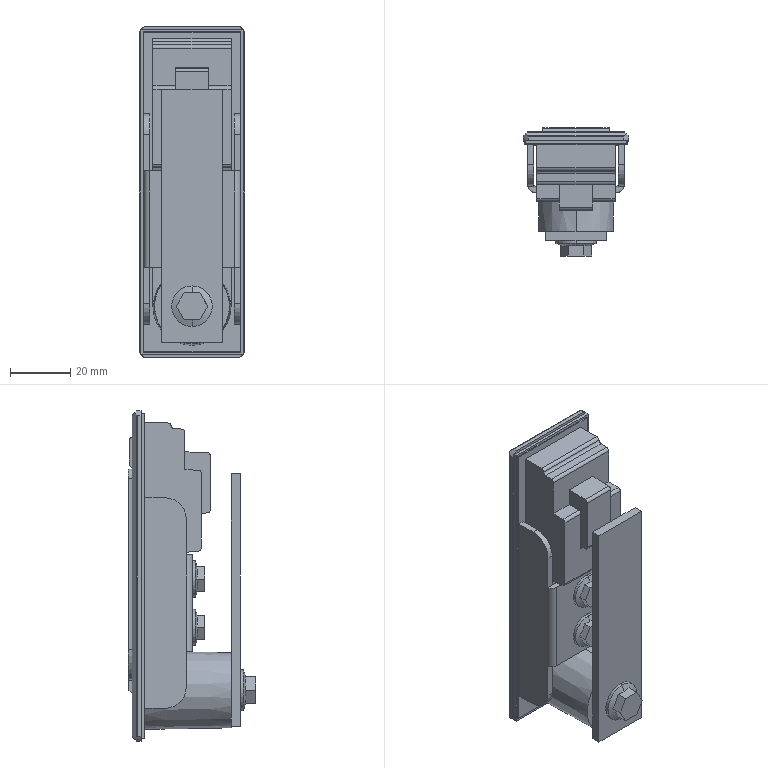Part | SolidWorks | features BaseBody 1 | 1 solid | 256 faces | box 35 x 42.5 x 110 mm | volume 68844 mm3 | plane 160 | cylinder 88 | cone 8 | commonest cylinder face diameters 2 x15 1 x9 12 x8 0.8 x4 4 x4 14 x4